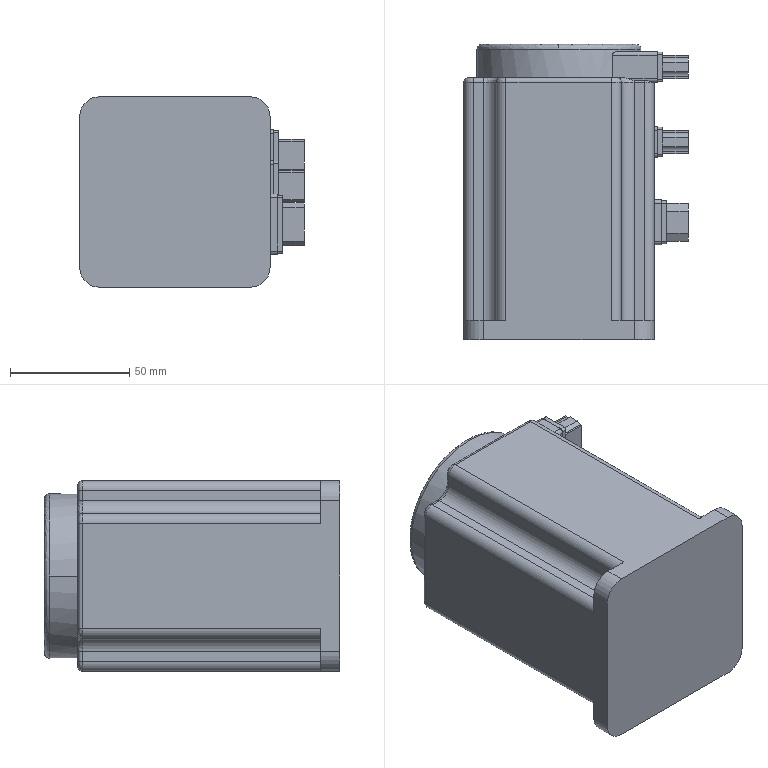Part | STEP file | Link3_J4mot | 1 solid | 154 faces | box 94.4 x 124 x 80 mm | volume 690172 mm3 | plane 77 | cylinder 63 | spline 10 | torus 4 | commonest cylinder face diameters 2 x12 3 x12 4 x12 8 x9 5 x8 11 x4